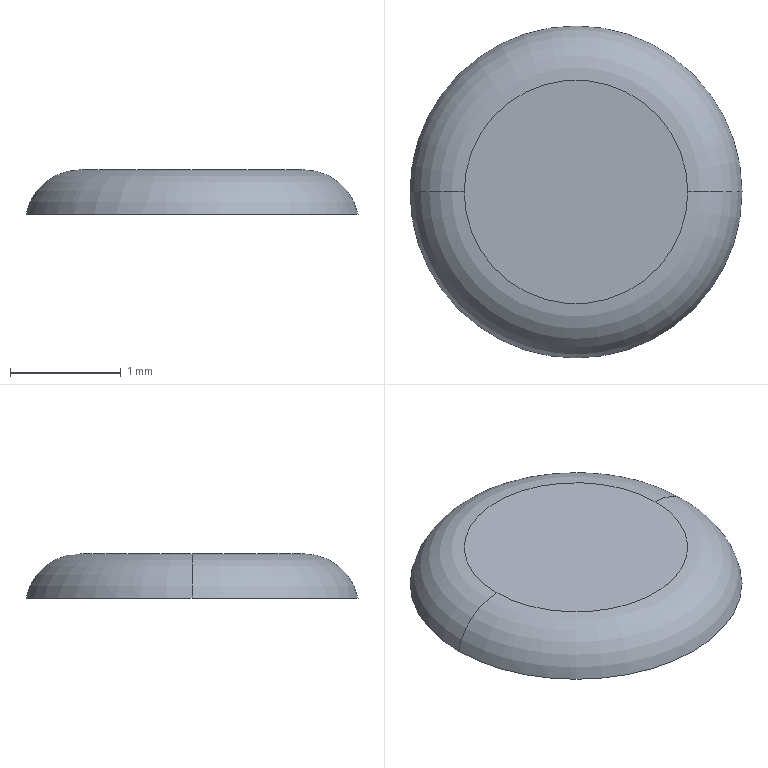Part | SolidWorks | features Extrusion 1, Fillet 1, Shell 1 | 1 solid | 7 faces | box 3 x 3 x 0.4 mm | volume 0.8046 mm3 | torus 4 | plane 3
STEP:
#1=CARTESIAN_POINT('',(-1.01,0.,0.1));
#2=VERTEX_POINT('',#1);
#3=CARTESIAN_POINT('',(1.01,0.,0.1));
#4=VERTEX_POINT('',#3);
#5=CARTESIAN_POINT('',(0.,0.,0.1));
#6=DIRECTION('',(0.,0.,1.));
#7=DIRECTION('',(-1.,0.,0.));
#8=AXIS2_PLACEMENT_3D('',#5,#6,#7);
#9=CIRCLE('',#8,1.01);
#10=EDGE_CURVE('',#2,#4,#9,.T.);
#11=ORIENTED_EDGE('',*,*,#10,.T.);
#12=CARTESIAN_POINT('',(1.397,0.,-0.2));
#13=VERTEX_POINT('',#12);
#14=CARTESIAN_POINT('',(1.01,0.,-0.3));
#15=DIRECTION('',(0.,1.,0.));
#16=DIRECTION('',(-1.,0.,0.));
#17=AXIS2_PLACEMENT_3D('',#14,#15,#16);
#18=CIRCLE('',#17,0.4);
#19=EDGE_CURVE('',#4,#13,#18,.T.);
#20=ORIENTED_EDGE('',*,*,#19,.T.);
#21=CARTESIAN_POINT('',(-1.397,0.,-0.2));
#22=VERTEX_POINT('',#21);
#23=CARTESIAN_POINT('',(0.,0.,-0.2));
#24=DIRECTION('',(0.,0.,1.));
#25=DIRECTION('',(1.,0.,0.));
#26=AXIS2_PLACEMENT_3D('',#23,#24,#25);
#27=CIRCLE('',#26,1.397);
#28=EDGE_CURVE('',#22,#13,#27,.T.);
#29=ORIENTED_EDGE('',*,*,#28,.F.);
#30=CARTESIAN_POINT('',(-1.01,0.,-0.3));
#31=DIRECTION('',(0.,-1.,0.));
#32=DIRECTION('',(0.,0.,-1.));
#33=AXIS2_PLACEMENT_3D('',#30,#31,#32);
#34=CIRCLE('',#33,0.4);
#35=EDGE_CURVE('',#2,#22,#34,.T.);
#36=ORIENTED_EDGE('',*,*,#35,.F.);
#37=EDGE_LOOP('',(#11,#20,#29,#36));
#38=FACE_OUTER_BOUND('',#37,.T.);
#39=CARTESIAN_POINT('',(0.,0.,-0.3));
#40=DIRECTION('',(0.,0.,-1.));
#41=DIRECTION('',(-1.,0.,0.));
#42=AXIS2_PLACEMENT_3D('',#39,#40,#41);
#43=TOROIDAL_SURFACE('',#42,1.01,0.4);
#44=ADVANCED_FACE('',(#38),#43,.F.);
#45=CARTESIAN_POINT('',(1.01,0.,0.2));
#46=VERTEX_POINT('',#45);
#47=CARTESIAN_POINT('',(-1.01,0.,0.2));
#48=VERTEX_POINT('',#47);
#49=CARTESIAN_POINT('',(0.,0.,0.2));
#50=DIRECTION('',(0.,0.,1.));
#51=DIRECTION('',(1.,0.,0.));
#52=AXIS2_PLACEMENT_3D('',#49,#50,#51);
#53=CIRCLE('',#52,1.01);
#54=EDGE_CURVE('',#46,#48,#53,.T.);
#55=ORIENTED_EDGE('',*,*,#54,.F.);
#56=CARTESIAN_POINT('',(1.5,0.,-0.2));
#57=VERTEX_POINT('',#56);
#58=CARTESIAN_POINT('',(1.01,0.,-0.3));
#59=DIRECTION('',(0.,1.,0.));
#60=DIRECTION('',(-1.,0.,0.));
#61=AXIS2_PLACEMENT_3D('',#58,#59,#60);
#62=CIRCLE('',#61,0.5);
#63=EDGE_CURVE('',#46,#57,#62,.T.);
#64=ORIENTED_EDGE('',*,*,#63,.T.);
#65=CARTESIAN_POINT('',(-1.5,0.,-0.2));
#66=VERTEX_POINT('',#65);
#67=CARTESIAN_POINT('',(0.,0.,-0.2));
#68=DIRECTION('',(0.,0.,1.));
#69=DIRECTION('',(1.,0.,0.));
#70=AXIS2_PLACEMENT_3D('',#67,#68,#69);
#71=CIRCLE('',#70,1.5);
#72=EDGE_CURVE('',#57,#66,#71,.T.);
#73=ORIENTED_EDGE('',*,*,#72,.T.);
#74=CARTESIAN_POINT('',(-1.01,0.,-0.3));
#75=DIRECTION('',(0.,-1.,0.));
#76=DIRECTION('',(0.,0.,-1.));
#77=AXIS2_PLACEMENT_3D('',#74,#75,#76);
#78=CIRCLE('',#77,0.5);
#79=EDGE_CURVE('',#48,#66,#78,.T.);
#80=ORIENTED_EDGE('',*,*,#79,.F.);
#81=EDGE_LOOP('',(#55,#64,#73,#80));
#82=FACE_OUTER_BOUND('',#81,.T.);
#83=CARTESIAN_POINT('',(0.,0.,-0.3));
#84=DIRECTION('',(0.,0.,-1.));
#85=DIRECTION('',(-1.,0.,0.));
#86=AXIS2_PLACEMENT_3D('',#83,#84,#85);
#87=TOROIDAL_SURFACE('',#86,1.01,0.5);
#88=ADVANCED_FACE('',(#82),#87,.T.);
#89=CARTESIAN_POINT('',(0.,0.,0.2));
#90=DIRECTION('',(0.,0.,1.));
#91=DIRECTION('',(1.,0.,0.));
#92=AXIS2_PLACEMENT_3D('',#89,#90,#91);
#93=CIRCLE('',#92,1.01);
#94=EDGE_CURVE('',#48,#46,#93,.T.);
#95=ORIENTED_EDGE('',*,*,#94,.T.);
#96=ORIENTED_EDGE('',*,*,#54,.T.);
#97=EDGE_LOOP('',(#95,#96));
#98=FACE_OUTER_BOUND('',#97,.T.);
#99=CARTESIAN_POINT('',(0.,0.,0.2));
#100=DIRECTION('',(0.,0.,1.));
#101=DIRECTION('',(1.,0.,0.));
#102=AXIS2_PLACEMENT_3D('',#99,#100,#101);
#103=PLANE('',#102);
#104=ADVANCED_FACE('',(#98),#103,.T.);
#105=ORIENTED_EDGE('',*,*,#28,.T.);
#106=CARTESIAN_POINT('',(0.,0.,-0.2));
#107=DIRECTION('',(0.,0.,1.));
#108=DIRECTION('',(1.,0.,0.));
#109=AXIS2_PLACEMENT_3D('',#106,#107,#108);
#110=CIRCLE('',#109,1.397);
#111=EDGE_CURVE('',#13,#22,#110,.T.);
#112=ORIENTED_EDGE('',*,*,#111,.T.);
#113=EDGE_LOOP('',(#105,#112));
#114=FACE_BOUND('',#113,.T.);
#115=CARTESIAN_POINT('',(0.,0.,-0.2));
#116=DIRECTION('',(0.,0.,1.));
#117=DIRECTION('',(1.,0.,0.));
#118=AXIS2_PLACEMENT_3D('',#115,#116,#117);
#119=CIRCLE('',#118,1.5);
#120=EDGE_CURVE('',#66,#57,#119,.T.);
#121=ORIENTED_EDGE('',*,*,#120,.F.);
#122=ORIENTED_EDGE('',*,*,#72,.F.);
#123=EDGE_LOOP('',(#121,#122));
#124=FACE_OUTER_BOUND('',#123,.T.);
#125=CARTESIAN_POINT('',(0.,0.,-0.2));
#126=DIRECTION('',(0.,0.,1.));
#127=DIRECTION('',(1.,0.,0.));
#128=AXIS2_PLACEMENT_3D('',#125,#126,#127);
#129=PLANE('',#128);
#130=ADVANCED_FACE('',(#114,#124),#129,.F.);
#131=ORIENTED_EDGE('',*,*,#63,.F.);
#132=ORIENTED_EDGE('',*,*,#94,.F.);
#133=ORIENTED_EDGE('',*,*,#79,.T.);
#134=ORIENTED_EDGE('',*,*,#120,.T.);
#135=EDGE_LOOP('',(#131,#132,#133,#134));
#136=FACE_OUTER_BOUND('',#135,.T.);
#137=CARTESIAN_POINT('',(0.,0.,-0.3));
#138=DIRECTION('',(0.,0.,-1.));
#139=DIRECTION('',(-1.,0.,0.));
#140=AXIS2_PLACEMENT_3D('',#137,#138,#139);
#141=TOROIDAL_SURFACE('',#140,1.01,0.5);
#142=ADVANCED_FACE('',(#136),#141,.T.);
#143=ORIENTED_EDGE('',*,*,#10,.F.);
#144=CARTESIAN_POINT('',(0.,0.,0.1));
#145=DIRECTION('',(0.,0.,1.));
#146=DIRECTION('',(-1.,0.,0.));
#147=AXIS2_PLACEMENT_3D('',#144,#145,#146);
#148=CIRCLE('',#147,1.01);
#149=EDGE_CURVE('',#4,#2,#148,.T.);
#150=ORIENTED_EDGE('',*,*,#149,.F.);
#151=EDGE_LOOP('',(#143,#150));
#152=FACE_OUTER_BOUND('',#151,.T.);
#153=CARTESIAN_POINT('',(0.,0.,0.1));
#154=DIRECTION('',(0.,0.,1.));
#155=DIRECTION('',(1.,0.,0.));
#156=AXIS2_PLACEMENT_3D('',#153,#154,#155);
#157=PLANE('',#156);
#158=ADVANCED_FACE('',(#152),#157,.F.);
#159=ORIENTED_EDGE('',*,*,#19,.F.);
#160=ORIENTED_EDGE('',*,*,#149,.T.);
#161=ORIENTED_EDGE('',*,*,#35,.T.);
#162=ORIENTED_EDGE('',*,*,#111,.F.);
#163=EDGE_LOOP('',(#159,#160,#161,#162));
#164=FACE_OUTER_BOUND('',#163,.T.);
#165=CARTESIAN_POINT('',(0.,0.,-0.3));
#166=DIRECTION('',(0.,0.,-1.));
#167=DIRECTION('',(-1.,0.,0.));
#168=AXIS2_PLACEMENT_3D('',#165,#166,#167);
#169=TOROIDAL_SURFACE('',#168,1.01,0.4);
#170=ADVANCED_FACE('',(#164),#169,.F.);
#171=CLOSED_SHELL('',(#44,#88,#104,#130,#142,#158,#170));
#172=MANIFOLD_SOLID_BREP('',#171);
#173=CARTESIAN_POINT('',(0.,0.,0.));
#174=DIRECTION('',(0.,0.,1.));
#175=DIRECTION('',(1.,0.,0.));
#176=AXIS2_PLACEMENT_3D('',#173,#174,#175);
#177=(LENGTH_UNIT()NAMED_UNIT(*)SI_UNIT(.MILLI.,.METRE.));
#178=UNCERTAINTY_MEASURE_WITH_UNIT(LENGTH_MEASURE(0.00001),#177,'','');
#179=(NAMED_UNIT(*)PLANE_ANGLE_UNIT()SI_UNIT($,.RADIAN.));
#180=(NAMED_UNIT(*)SI_UNIT($,.STERADIAN.)SOLID_ANGLE_UNIT());
#181=(GEOMETRIC_REPRESENTATION_CONTEXT(3)GLOBAL_UNCERTAINTY_ASSIGNED_CONTEXT((#178))GLOBAL_UNIT_ASSIGNED_CONTEXT((#177,#179,#180))REPRESENTATION_CONTEXT('',''));
#182=ADVANCED_BREP_SHAPE_REPRESENTATION('',(#172,#176),#181);